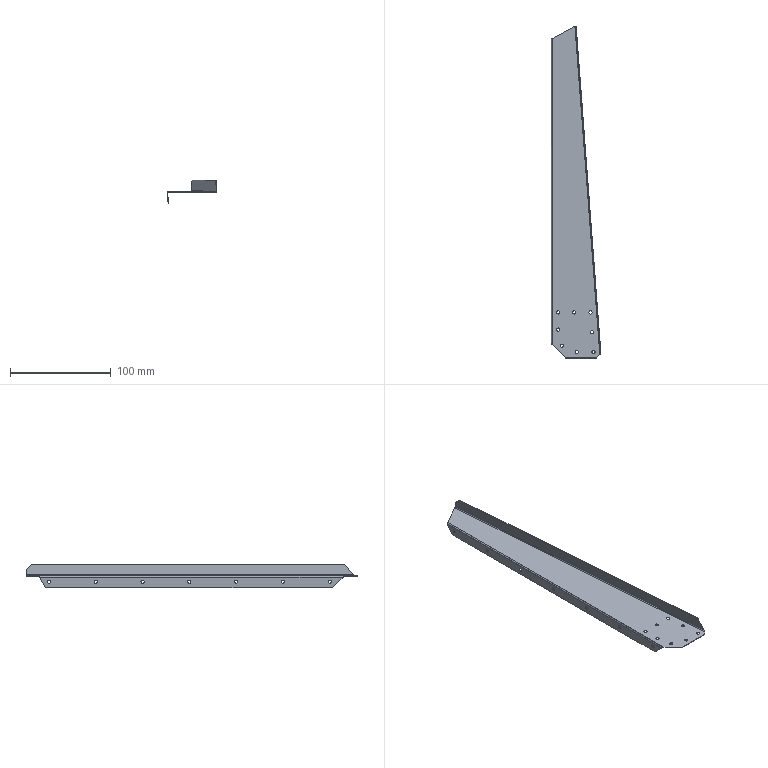Part | SolidWorks | features BaseBody 1 | 1 solid | 56 faces | box 49.549 x 330.007 x 23.452 mm | volume 9367 mm3 | cylinder 34 | plane 17 | spline 5 | commonest cylinder face diameters 3.2 x30 1.5 x2 2.5 x2